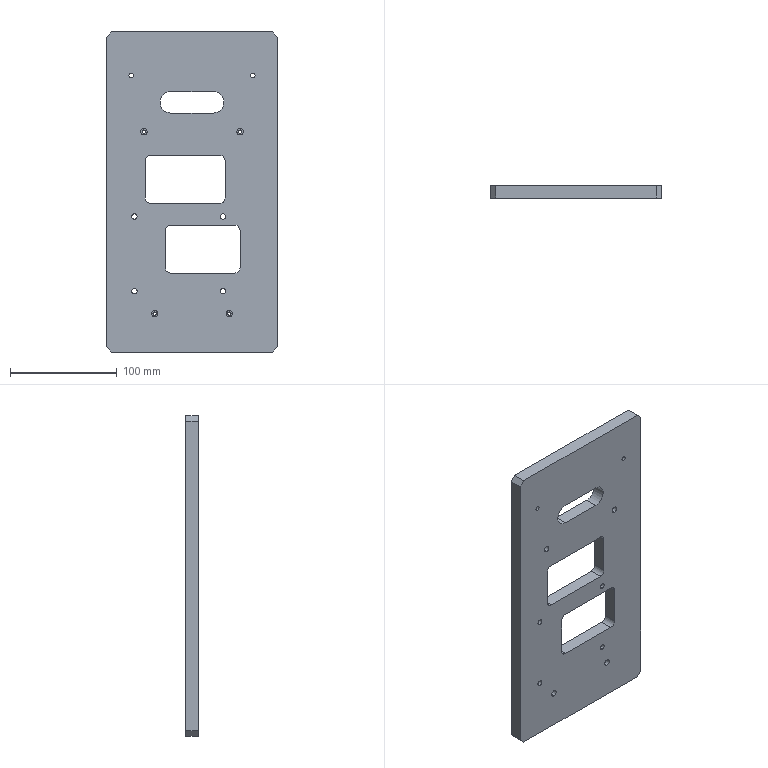Part | SolidWorks | features HoleWzd 12, ICE 6, Chamfer 1, Extrusion 1, Fillet 1, MirrorPattern 1 | 1 solid | 62 faces | box 160 x 12 x 300 mm | volume 482018 mm3 | cylinder 38 | plane 24 | commonest cylinder face diameters 3.2 x8 5 x8 6 x8 10 x8 4.2 x4 20 x2